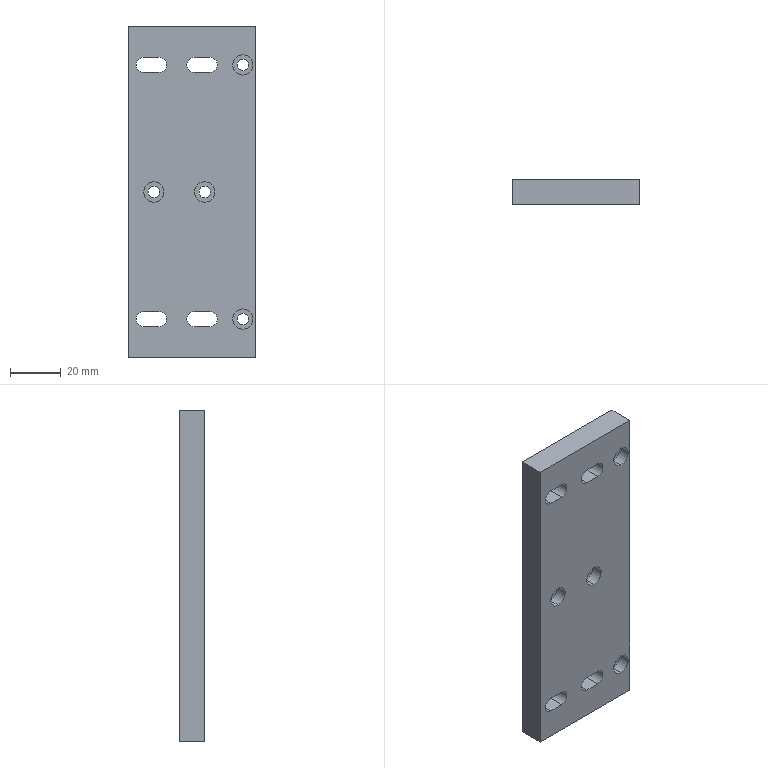Part | STEP file | 0243_206_Plate | 1 solid | 42 faces | box 50 x 10 x 130 mm | volume 61174 mm3 | cylinder 24 | plane 18 | commonest cylinder face diameters 4.5 x8 6 x8 8 x8